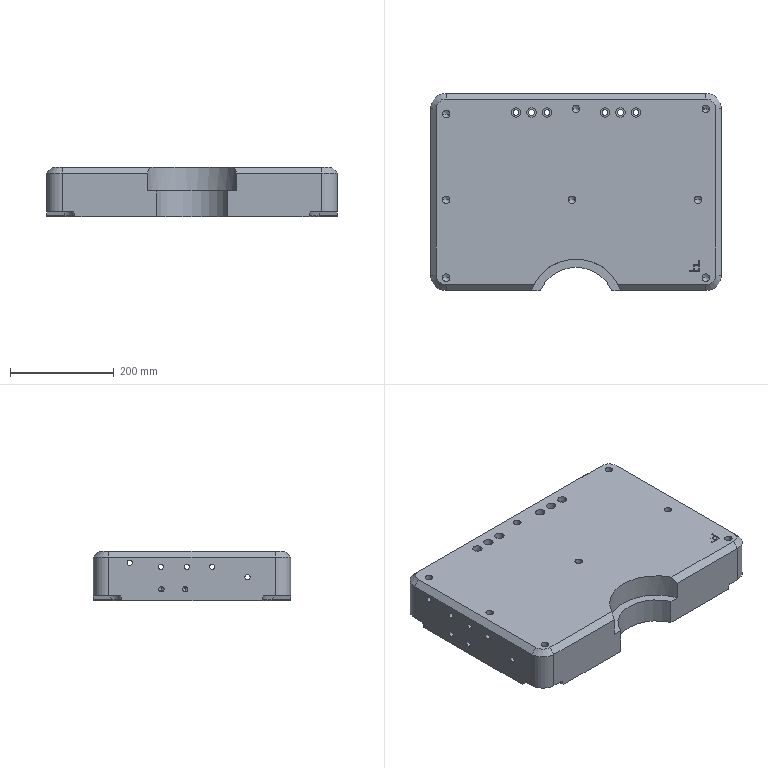Part | SolidWorks | features BaseBody 1 | 1 solid | 414 faces | box 560 x 380 x 95 mm | volume 14634768 mm3 | cylinder 149 | plane 85 | cone 72 | torus 69 | spline 37 | sphere 2 | commonest cylinder face diameters 4 x24 14.5 x20 2.011 x19 6.033 x15 10 x15 11 x12